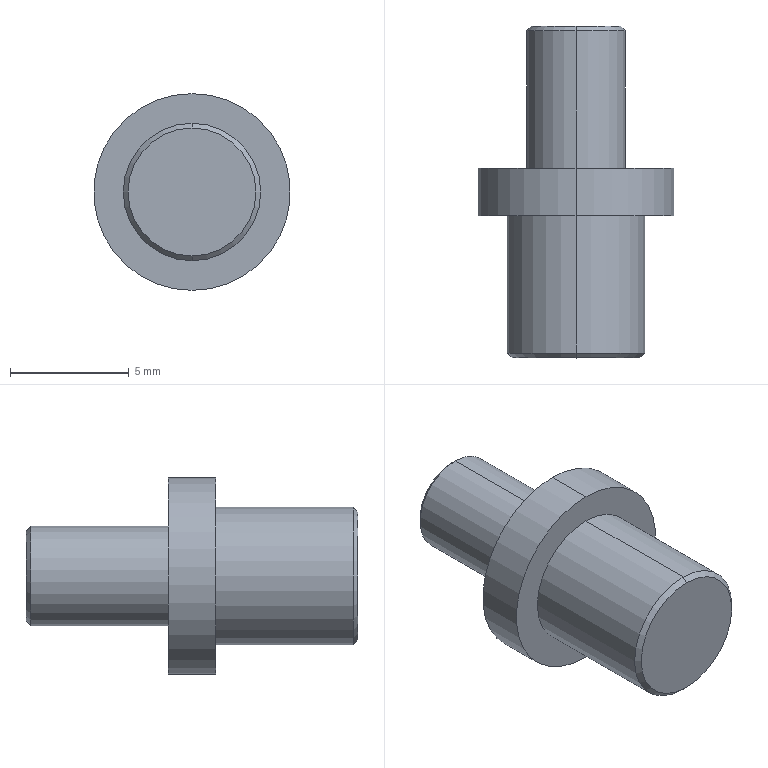Part | SolidWorks | features Chamfer 1, Revolution 1 | 1 solid | 14 faces | box 8.3 x 14 x 8.3 mm | volume 349.252 mm3 | cylinder 6 | cone 4 | plane 4 | commonest cylinder face diameters 4.2 x2 5.8 x2 8.3 x2
STEP:
#1=CARTESIAN_POINT('',(0.,14.,1.9));
#2=VERTEX_POINT('',#1);
#3=CARTESIAN_POINT('',(0.,14.,-1.9));
#4=VERTEX_POINT('',#3);
#5=CARTESIAN_POINT('',(0.,14.,0.));
#6=DIRECTION('',(0.,1.,0.));
#7=DIRECTION('',(0.,0.,1.));
#8=AXIS2_PLACEMENT_3D('',#5,#6,#7);
#9=CIRCLE('',#8,1.9);
#10=EDGE_CURVE('',#2,#4,#9,.T.);
#11=ORIENTED_EDGE('',*,*,#10,.F.);
#12=CARTESIAN_POINT('',(0.,13.8,2.1));
#13=VERTEX_POINT('',#12);
#14=CARTESIAN_POINT('',(0.,13.8,2.1));
#15=DIRECTION('',(0.,-0.7071,0.7071));
#16=VECTOR('',#15,1000.);
#17=LINE('',#14,#16);
#18=EDGE_CURVE('',#2,#13,#17,.T.);
#19=ORIENTED_EDGE('',*,*,#18,.T.);
#20=CARTESIAN_POINT('',(0.,13.8,-2.1));
#21=VERTEX_POINT('',#20);
#22=CARTESIAN_POINT('',(0.,13.8,0.));
#23=DIRECTION('',(0.,-1.,0.));
#24=DIRECTION('',(0.,0.,1.));
#25=AXIS2_PLACEMENT_3D('',#22,#23,#24);
#26=CIRCLE('',#25,2.1);
#27=EDGE_CURVE('',#21,#13,#26,.T.);
#28=ORIENTED_EDGE('',*,*,#27,.F.);
#29=CARTESIAN_POINT('',(0.,13.8,-2.1));
#30=DIRECTION('',(0.,-0.7071,-0.7071));
#31=VECTOR('',#30,1000.);
#32=LINE('',#29,#31);
#33=EDGE_CURVE('',#4,#21,#32,.T.);
#34=ORIENTED_EDGE('',*,*,#33,.F.);
#35=EDGE_LOOP('',(#11,#19,#28,#34));
#36=FACE_OUTER_BOUND('',#35,.T.);
#37=CARTESIAN_POINT('',(0.,13.8,0.));
#38=DIRECTION('',(0.,-1.,0.));
#39=DIRECTION('',(0.,0.,-1.));
#40=AXIS2_PLACEMENT_3D('',#37,#38,#39);
#41=CONICAL_SURFACE('',#40,2.1,0.7854);
#42=ADVANCED_FACE('',(#36),#41,.T.);
#43=CARTESIAN_POINT('',(0.,0.,-2.7));
#44=VERTEX_POINT('',#43);
#45=CARTESIAN_POINT('',(0.,0.,2.7));
#46=VERTEX_POINT('',#45);
#47=CARTESIAN_POINT('',(0.,0.,0.));
#48=DIRECTION('',(0.,-1.,0.));
#49=DIRECTION('',(0.,0.,-1.));
#50=AXIS2_PLACEMENT_3D('',#47,#48,#49);
#51=CIRCLE('',#50,2.7);
#52=EDGE_CURVE('',#44,#46,#51,.T.);
#53=ORIENTED_EDGE('',*,*,#52,.F.);
#54=CARTESIAN_POINT('',(0.,0.2,-2.9));
#55=VERTEX_POINT('',#54);
#56=CARTESIAN_POINT('',(0.,0.,-2.7));
#57=DIRECTION('',(0.,0.7071,-0.7071));
#58=VECTOR('',#57,1000.);
#59=LINE('',#56,#58);
#60=EDGE_CURVE('',#44,#55,#59,.T.);
#61=ORIENTED_EDGE('',*,*,#60,.T.);
#62=CARTESIAN_POINT('',(0.,0.2,2.9));
#63=VERTEX_POINT('',#62);
#64=CARTESIAN_POINT('',(0.,0.2,0.));
#65=DIRECTION('',(0.,1.,0.));
#66=DIRECTION('',(0.,0.,-1.));
#67=AXIS2_PLACEMENT_3D('',#64,#65,#66);
#68=CIRCLE('',#67,2.9);
#69=EDGE_CURVE('',#63,#55,#68,.T.);
#70=ORIENTED_EDGE('',*,*,#69,.F.);
#71=CARTESIAN_POINT('',(0.,0.,2.7));
#72=DIRECTION('',(0.,0.7071,0.7071));
#73=VECTOR('',#72,1000.);
#74=LINE('',#71,#73);
#75=EDGE_CURVE('',#46,#63,#74,.T.);
#76=ORIENTED_EDGE('',*,*,#75,.F.);
#77=EDGE_LOOP('',(#53,#61,#70,#76));
#78=FACE_OUTER_BOUND('',#77,.T.);
#79=CARTESIAN_POINT('',(0.,0.,0.));
#80=DIRECTION('',(0.,1.,0.));
#81=DIRECTION('',(0.,0.,1.));
#82=AXIS2_PLACEMENT_3D('',#79,#80,#81);
#83=CONICAL_SURFACE('',#82,2.7,0.7854);
#84=ADVANCED_FACE('',(#78),#83,.T.);
#85=ORIENTED_EDGE('',*,*,#27,.T.);
#86=CARTESIAN_POINT('',(0.,8.,2.1));
#87=VERTEX_POINT('',#86);
#88=CARTESIAN_POINT('',(0.,0.,2.1));
#89=DIRECTION('',(0.,-1.,0.));
#90=VECTOR('',#89,1000.);
#91=LINE('',#88,#90);
#92=EDGE_CURVE('',#13,#87,#91,.T.);
#93=ORIENTED_EDGE('',*,*,#92,.T.);
#94=CARTESIAN_POINT('',(0.,8.,-2.1));
#95=VERTEX_POINT('',#94);
#96=CARTESIAN_POINT('',(0.,8.,0.));
#97=DIRECTION('',(0.,-1.,0.));
#98=DIRECTION('',(0.,0.,-1.));
#99=AXIS2_PLACEMENT_3D('',#96,#97,#98);
#100=CIRCLE('',#99,2.1);
#101=EDGE_CURVE('',#95,#87,#100,.T.);
#102=ORIENTED_EDGE('',*,*,#101,.F.);
#103=CARTESIAN_POINT('',(0.,0.,-2.1));
#104=DIRECTION('',(0.,-1.,0.));
#105=VECTOR('',#104,1000.);
#106=LINE('',#103,#105);
#107=EDGE_CURVE('',#21,#95,#106,.T.);
#108=ORIENTED_EDGE('',*,*,#107,.F.);
#109=EDGE_LOOP('',(#85,#93,#102,#108));
#110=FACE_OUTER_BOUND('',#109,.T.);
#111=CARTESIAN_POINT('',(0.,0.,0.));
#112=DIRECTION('',(0.,-1.,0.));
#113=DIRECTION('',(0.,0.,-1.));
#114=AXIS2_PLACEMENT_3D('',#111,#112,#113);
#115=CYLINDRICAL_SURFACE('',#114,2.1);
#116=ADVANCED_FACE('',(#110),#115,.T.);
#117=CARTESIAN_POINT('',(0.,8.,-4.15));
#118=VERTEX_POINT('',#117);
#119=CARTESIAN_POINT('',(0.,8.,4.15));
#120=VERTEX_POINT('',#119);
#121=CARTESIAN_POINT('',(0.,8.,0.));
#122=DIRECTION('',(0.,-1.,0.));
#123=DIRECTION('',(0.,0.,-1.));
#124=AXIS2_PLACEMENT_3D('',#121,#122,#123);
#125=CIRCLE('',#124,4.15);
#126=EDGE_CURVE('',#118,#120,#125,.T.);
#127=ORIENTED_EDGE('',*,*,#126,.T.);
#128=CARTESIAN_POINT('',(0.,6.,4.15));
#129=VERTEX_POINT('',#128);
#130=CARTESIAN_POINT('',(0.,0.,4.15));
#131=DIRECTION('',(0.,-1.,0.));
#132=VECTOR('',#131,1000.);
#133=LINE('',#130,#132);
#134=EDGE_CURVE('',#120,#129,#133,.T.);
#135=ORIENTED_EDGE('',*,*,#134,.T.);
#136=CARTESIAN_POINT('',(0.,6.,-4.15));
#137=VERTEX_POINT('',#136);
#138=CARTESIAN_POINT('',(0.,6.,0.));
#139=DIRECTION('',(0.,-1.,0.));
#140=DIRECTION('',(0.,0.,-1.));
#141=AXIS2_PLACEMENT_3D('',#138,#139,#140);
#142=CIRCLE('',#141,4.15);
#143=EDGE_CURVE('',#137,#129,#142,.T.);
#144=ORIENTED_EDGE('',*,*,#143,.F.);
#145=CARTESIAN_POINT('',(0.,0.,-4.15));
#146=DIRECTION('',(0.,-1.,0.));
#147=VECTOR('',#146,1000.);
#148=LINE('',#145,#147);
#149=EDGE_CURVE('',#118,#137,#148,.T.);
#150=ORIENTED_EDGE('',*,*,#149,.F.);
#151=EDGE_LOOP('',(#127,#135,#144,#150));
#152=FACE_OUTER_BOUND('',#151,.T.);
#153=CARTESIAN_POINT('',(0.,0.,0.));
#154=DIRECTION('',(0.,-1.,0.));
#155=DIRECTION('',(0.,0.,-1.));
#156=AXIS2_PLACEMENT_3D('',#153,#154,#155);
#157=CYLINDRICAL_SURFACE('',#156,4.15);
#158=ADVANCED_FACE('',(#152),#157,.T.);
#159=CARTESIAN_POINT('',(0.,6.,-2.9));
#160=VERTEX_POINT('',#159);
#161=CARTESIAN_POINT('',(0.,6.,2.9));
#162=VERTEX_POINT('',#161);
#163=CARTESIAN_POINT('',(0.,6.,0.));
#164=DIRECTION('',(0.,-1.,0.));
#165=DIRECTION('',(0.,0.,-1.));
#166=AXIS2_PLACEMENT_3D('',#163,#164,#165);
#167=CIRCLE('',#166,2.9);
#168=EDGE_CURVE('',#160,#162,#167,.T.);
#169=ORIENTED_EDGE('',*,*,#168,.T.);
#170=CARTESIAN_POINT('',(0.,0.,2.9));
#171=DIRECTION('',(0.,-1.,0.));
#172=VECTOR('',#171,1000.);
#173=LINE('',#170,#172);
#174=EDGE_CURVE('',#162,#63,#173,.T.);
#175=ORIENTED_EDGE('',*,*,#174,.T.);
#176=ORIENTED_EDGE('',*,*,#69,.T.);
#177=CARTESIAN_POINT('',(0.,0.,-2.9));
#178=DIRECTION('',(0.,-1.,0.));
#179=VECTOR('',#178,1000.);
#180=LINE('',#177,#179);
#181=EDGE_CURVE('',#160,#55,#180,.T.);
#182=ORIENTED_EDGE('',*,*,#181,.F.);
#183=EDGE_LOOP('',(#169,#175,#176,#182));
#184=FACE_OUTER_BOUND('',#183,.T.);
#185=CARTESIAN_POINT('',(0.,0.,0.));
#186=DIRECTION('',(0.,-1.,0.));
#187=DIRECTION('',(0.,0.,-1.));
#188=AXIS2_PLACEMENT_3D('',#185,#186,#187);
#189=CYLINDRICAL_SURFACE('',#188,2.9);
#190=ADVANCED_FACE('',(#184),#189,.T.);
#191=CARTESIAN_POINT('',(0.,0.,0.));
#192=DIRECTION('',(0.,-1.,0.));
#193=DIRECTION('',(0.,0.,-1.));
#194=AXIS2_PLACEMENT_3D('',#191,#192,#193);
#195=CIRCLE('',#194,2.7);
#196=EDGE_CURVE('',#46,#44,#195,.T.);
#197=ORIENTED_EDGE('',*,*,#196,.T.);
#198=ORIENTED_EDGE('',*,*,#52,.T.);
#199=EDGE_LOOP('',(#197,#198));
#200=FACE_OUTER_BOUND('',#199,.T.);
#201=CARTESIAN_POINT('',(0.,0.,0.));
#202=DIRECTION('',(0.,-1.,0.));
#203=DIRECTION('',(0.,0.,-1.));
#204=AXIS2_PLACEMENT_3D('',#201,#202,#203);
#205=PLANE('',#204);
#206=ADVANCED_FACE('',(#200),#205,.T.);
#207=ORIENTED_EDGE('',*,*,#174,.F.);
#208=CARTESIAN_POINT('',(0.,6.,0.));
#209=DIRECTION('',(0.,-1.,0.));
#210=DIRECTION('',(0.,0.,-1.));
#211=AXIS2_PLACEMENT_3D('',#208,#209,#210);
#212=CIRCLE('',#211,2.9);
#213=EDGE_CURVE('',#162,#160,#212,.T.);
#214=ORIENTED_EDGE('',*,*,#213,.T.);
#215=ORIENTED_EDGE('',*,*,#181,.T.);
#216=CARTESIAN_POINT('',(0.,0.2,0.));
#217=DIRECTION('',(0.,1.,0.));
#218=DIRECTION('',(0.,0.,-1.));
#219=AXIS2_PLACEMENT_3D('',#216,#217,#218);
#220=CIRCLE('',#219,2.9);
#221=EDGE_CURVE('',#55,#63,#220,.T.);
#222=ORIENTED_EDGE('',*,*,#221,.T.);
#223=EDGE_LOOP('',(#207,#214,#215,#222));
#224=FACE_OUTER_BOUND('',#223,.T.);
#225=CARTESIAN_POINT('',(0.,0.,0.));
#226=DIRECTION('',(0.,-1.,0.));
#227=DIRECTION('',(0.,0.,-1.));
#228=AXIS2_PLACEMENT_3D('',#225,#226,#227);
#229=CYLINDRICAL_SURFACE('',#228,2.9);
#230=ADVANCED_FACE('',(#224),#229,.T.);
#231=ORIENTED_EDGE('',*,*,#143,.T.);
#232=CARTESIAN_POINT('',(0.,6.,0.));
#233=DIRECTION('',(0.,-1.,0.));
#234=DIRECTION('',(0.,0.,-1.));
#235=AXIS2_PLACEMENT_3D('',#232,#233,#234);
#236=CIRCLE('',#235,4.15);
#237=EDGE_CURVE('',#129,#137,#236,.T.);
#238=ORIENTED_EDGE('',*,*,#237,.T.);
#239=EDGE_LOOP('',(#231,#238));
#240=FACE_OUTER_BOUND('',#239,.T.);
#241=ORIENTED_EDGE('',*,*,#168,.F.);
#242=ORIENTED_EDGE('',*,*,#213,.F.);
#243=EDGE_LOOP('',(#241,#242));
#244=FACE_BOUND('',#243,.T.);
#245=CARTESIAN_POINT('',(2.9,6.,0.));
#246=DIRECTION('',(0.,-1.,0.));
#247=DIRECTION('',(0.,0.,-1.));
#248=AXIS2_PLACEMENT_3D('',#245,#246,#247);
#249=PLANE('',#248);
#250=ADVANCED_FACE('',(#240,#244),#249,.T.);
#251=ORIENTED_EDGE('',*,*,#134,.F.);
#252=CARTESIAN_POINT('',(0.,8.,0.));
#253=DIRECTION('',(0.,-1.,0.));
#254=DIRECTION('',(0.,0.,-1.));
#255=AXIS2_PLACEMENT_3D('',#252,#253,#254);
#256=CIRCLE('',#255,4.15);
#257=EDGE_CURVE('',#120,#118,#256,.T.);
#258=ORIENTED_EDGE('',*,*,#257,.T.);
#259=ORIENTED_EDGE('',*,*,#149,.T.);
#260=ORIENTED_EDGE('',*,*,#237,.F.);
#261=EDGE_LOOP('',(#251,#258,#259,#260));
#262=FACE_OUTER_BOUND('',#261,.T.);
#263=CARTESIAN_POINT('',(0.,0.,0.));
#264=DIRECTION('',(0.,-1.,0.));
#265=DIRECTION('',(0.,0.,-1.));
#266=AXIS2_PLACEMENT_3D('',#263,#264,#265);
#267=CYLINDRICAL_SURFACE('',#266,4.15);
#268=ADVANCED_FACE('',(#262),#267,.T.);
#269=ORIENTED_EDGE('',*,*,#101,.T.);
#270=CARTESIAN_POINT('',(0.,8.,0.));
#271=DIRECTION('',(0.,-1.,0.));
#272=DIRECTION('',(0.,0.,-1.));
#273=AXIS2_PLACEMENT_3D('',#270,#271,#272);
#274=CIRCLE('',#273,2.1);
#275=EDGE_CURVE('',#87,#95,#274,.T.);
#276=ORIENTED_EDGE('',*,*,#275,.T.);
#277=EDGE_LOOP('',(#269,#276));
#278=FACE_BOUND('',#277,.T.);
#279=ORIENTED_EDGE('',*,*,#126,.F.);
#280=ORIENTED_EDGE('',*,*,#257,.F.);
#281=EDGE_LOOP('',(#279,#280));
#282=FACE_OUTER_BOUND('',#281,.T.);
#283=CARTESIAN_POINT('',(4.15,8.,0.));
#284=DIRECTION('',(0.,1.,0.));
#285=DIRECTION('',(0.,0.,1.));
#286=AXIS2_PLACEMENT_3D('',#283,#284,#285);
#287=PLANE('',#286);
#288=ADVANCED_FACE('',(#278,#282),#287,.T.);
#289=ORIENTED_EDGE('',*,*,#92,.F.);
#290=CARTESIAN_POINT('',(0.,13.8,0.));
#291=DIRECTION('',(0.,-1.,0.));
#292=DIRECTION('',(0.,0.,1.));
#293=AXIS2_PLACEMENT_3D('',#290,#291,#292);
#294=CIRCLE('',#293,2.1);
#295=EDGE_CURVE('',#13,#21,#294,.T.);
#296=ORIENTED_EDGE('',*,*,#295,.T.);
#297=ORIENTED_EDGE('',*,*,#107,.T.);
#298=ORIENTED_EDGE('',*,*,#275,.F.);
#299=EDGE_LOOP('',(#289,#296,#297,#298));
#300=FACE_OUTER_BOUND('',#299,.T.);
#301=CARTESIAN_POINT('',(0.,0.,0.));
#302=DIRECTION('',(0.,-1.,0.));
#303=DIRECTION('',(0.,0.,-1.));
#304=AXIS2_PLACEMENT_3D('',#301,#302,#303);
#305=CYLINDRICAL_SURFACE('',#304,2.1);
#306=ADVANCED_FACE('',(#300),#305,.T.);
#307=CARTESIAN_POINT('',(0.,14.,0.));
#308=DIRECTION('',(0.,1.,0.));
#309=DIRECTION('',(0.,0.,1.));
#310=AXIS2_PLACEMENT_3D('',#307,#308,#309);
#311=CIRCLE('',#310,1.9);
#312=EDGE_CURVE('',#4,#2,#311,.T.);
#313=ORIENTED_EDGE('',*,*,#312,.T.);
#314=ORIENTED_EDGE('',*,*,#10,.T.);
#315=EDGE_LOOP('',(#313,#314));
#316=FACE_OUTER_BOUND('',#315,.T.);
#317=CARTESIAN_POINT('',(2.1,14.,0.));
#318=DIRECTION('',(0.,1.,0.));
#319=DIRECTION('',(0.,0.,1.));
#320=AXIS2_PLACEMENT_3D('',#317,#318,#319);
#321=PLANE('',#320);
#322=ADVANCED_FACE('',(#316),#321,.T.);
#323=ORIENTED_EDGE('',*,*,#60,.F.);
#324=ORIENTED_EDGE('',*,*,#196,.F.);
#325=ORIENTED_EDGE('',*,*,#75,.T.);
#326=ORIENTED_EDGE('',*,*,#221,.F.);
#327=EDGE_LOOP('',(#323,#324,#325,#326));
#328=FACE_OUTER_BOUND('',#327,.T.);
#329=CARTESIAN_POINT('',(0.,0.,0.));
#330=DIRECTION('',(0.,1.,0.));
#331=DIRECTION('',(0.,0.,1.));
#332=AXIS2_PLACEMENT_3D('',#329,#330,#331);
#333=CONICAL_SURFACE('',#332,2.7,0.7854);
#334=ADVANCED_FACE('',(#328),#333,.T.);
#335=ORIENTED_EDGE('',*,*,#18,.F.);
#336=ORIENTED_EDGE('',*,*,#312,.F.);
#337=ORIENTED_EDGE('',*,*,#33,.T.);
#338=ORIENTED_EDGE('',*,*,#295,.F.);
#339=EDGE_LOOP('',(#335,#336,#337,#338));
#340=FACE_OUTER_BOUND('',#339,.T.);
#341=CARTESIAN_POINT('',(0.,13.8,0.));
#342=DIRECTION('',(0.,-1.,0.));
#343=DIRECTION('',(0.,0.,-1.));
#344=AXIS2_PLACEMENT_3D('',#341,#342,#343);
#345=CONICAL_SURFACE('',#344,2.1,0.7854);
#346=ADVANCED_FACE('',(#340),#345,.T.);
#347=CLOSED_SHELL('',(#42,#84,#116,#158,#190,#206,#230,#250,#268,#288,#306,#322,#334,#346));
#348=MANIFOLD_SOLID_BREP('',#347);
#349=CARTESIAN_POINT('',(0.,0.,0.));
#350=DIRECTION('',(0.,0.,1.));
#351=DIRECTION('',(1.,0.,0.));
#352=AXIS2_PLACEMENT_3D('',#349,#350,#351);
#353=(LENGTH_UNIT()NAMED_UNIT(*)SI_UNIT(.MILLI.,.METRE.));
#354=UNCERTAINTY_MEASURE_WITH_UNIT(LENGTH_MEASURE(0.00001),#353,'','');
#355=(NAMED_UNIT(*)PLANE_ANGLE_UNIT()SI_UNIT($,.RADIAN.));
#356=(NAMED_UNIT(*)SI_UNIT($,.STERADIAN.)SOLID_ANGLE_UNIT());
#357=(GEOMETRIC_REPRESENTATION_CONTEXT(3)GLOBAL_UNCERTAINTY_ASSIGNED_CONTEXT((#354))GLOBAL_UNIT_ASSIGNED_CONTEXT((#353,#355,#356))REPRESENTATION_CONTEXT('',''));
#358=ADVANCED_BREP_SHAPE_REPRESENTATION('',(#348,#352),#357);